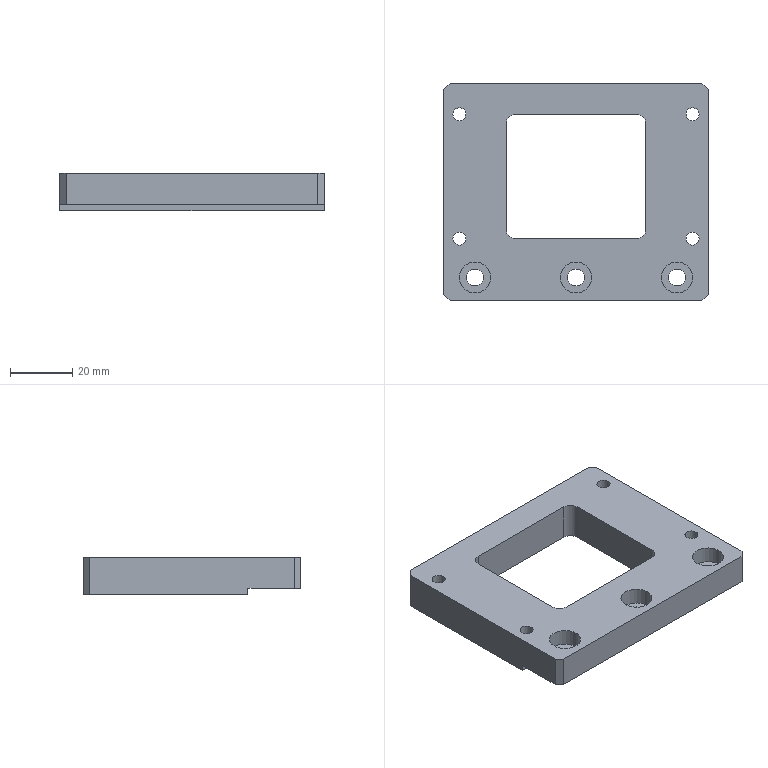Part | NX | 1 solid | 33 faces | box 85 x 70 x 12 mm | volume 44649 mm3 | plane 19 | cylinder 14 | commonest cylinder face diameters 4.2 x4 6 x4 5.5 x3 10 x3
STEP:
#1=CARTESIAN_POINT('',(-37.5,-27.5,0.6));
#2=VERTEX_POINT('',#1);
#3=CARTESIAN_POINT('',(-32.5,-27.5,0.6));
#4=DIRECTION('',(0.,0.,1.));
#5=DIRECTION('',(-1.,0.,0.));
#6=AXIS2_PLACEMENT_3D('',#3,#4,#5);
#7=CIRCLE('',#6,5.);
#8=EDGE_CURVE('',#2,#2,#7,.T.);
#9=ORIENTED_EDGE('',*,*,#8,.T.);
#10=EDGE_LOOP('',(#9));
#11=FACE_BOUND('',#10,.T.);
#12=CARTESIAN_POINT('',(-35.25,-27.5,0.6));
#13=VERTEX_POINT('',#12);
#14=CARTESIAN_POINT('',(-32.5,-27.5,0.6));
#15=DIRECTION('',(0.,0.,1.));
#16=DIRECTION('',(-1.,0.,0.));
#17=AXIS2_PLACEMENT_3D('',#14,#15,#16);
#18=CIRCLE('',#17,2.75);
#19=EDGE_CURVE('',#13,#13,#18,.T.);
#20=ORIENTED_EDGE('',*,*,#19,.F.);
#21=EDGE_LOOP('',(#20));
#22=FACE_BOUND('',#21,.T.);
#23=CARTESIAN_POINT('',(2.75,-27.5,0.6));
#24=DIRECTION('',(0.,0.,-1.));
#25=DIRECTION('',(-1.,0.,0.));
#26=AXIS2_PLACEMENT_3D('',#23,#24,#25);
#27=PLANE('',#26);
#28=ADVANCED_FACE('',(#11,#22),#27,.F.);
#29=CARTESIAN_POINT('',(5.,-27.5,0.6));
#30=VERTEX_POINT('',#29);
#31=CARTESIAN_POINT('',(0.,-27.5,0.6));
#32=DIRECTION('',(0.,0.,1.));
#33=DIRECTION('',(1.,0.,0.));
#34=AXIS2_PLACEMENT_3D('',#31,#32,#33);
#35=CIRCLE('',#34,5.);
#36=EDGE_CURVE('',#30,#30,#35,.T.);
#37=ORIENTED_EDGE('',*,*,#36,.T.);
#38=EDGE_LOOP('',(#37));
#39=FACE_BOUND('',#38,.T.);
#40=CARTESIAN_POINT('',(2.75,-27.5,0.6));
#41=VERTEX_POINT('',#40);
#42=CARTESIAN_POINT('',(0.,-27.5,0.6));
#43=DIRECTION('',(0.,0.,1.));
#44=DIRECTION('',(1.,0.,0.));
#45=AXIS2_PLACEMENT_3D('',#42,#43,#44);
#46=CIRCLE('',#45,2.75);
#47=EDGE_CURVE('',#41,#41,#46,.T.);
#48=ORIENTED_EDGE('',*,*,#47,.F.);
#49=EDGE_LOOP('',(#48));
#50=FACE_BOUND('',#49,.T.);
#51=CARTESIAN_POINT('',(2.75,-27.5,0.6));
#52=DIRECTION('',(0.,0.,-1.));
#53=DIRECTION('',(-1.,0.,0.));
#54=AXIS2_PLACEMENT_3D('',#51,#52,#53);
#55=PLANE('',#54);
#56=ADVANCED_FACE('',(#39,#50),#55,.F.);
#57=CARTESIAN_POINT('',(27.5,-27.5,0.6));
#58=VERTEX_POINT('',#57);
#59=CARTESIAN_POINT('',(32.5,-27.5,0.6));
#60=DIRECTION('',(0.,0.,1.));
#61=DIRECTION('',(-1.,0.,0.));
#62=AXIS2_PLACEMENT_3D('',#59,#60,#61);
#63=CIRCLE('',#62,5.);
#64=EDGE_CURVE('',#58,#58,#63,.T.);
#65=ORIENTED_EDGE('',*,*,#64,.T.);
#66=EDGE_LOOP('',(#65));
#67=FACE_BOUND('',#66,.T.);
#68=CARTESIAN_POINT('',(29.75,-27.5,0.6));
#69=VERTEX_POINT('',#68);
#70=CARTESIAN_POINT('',(32.5,-27.5,0.6));
#71=DIRECTION('',(0.,0.,1.));
#72=DIRECTION('',(-1.,0.,0.));
#73=AXIS2_PLACEMENT_3D('',#70,#71,#72);
#74=CIRCLE('',#73,2.75);
#75=EDGE_CURVE('',#69,#69,#74,.T.);
#76=ORIENTED_EDGE('',*,*,#75,.F.);
#77=EDGE_LOOP('',(#76));
#78=FACE_BOUND('',#77,.T.);
#79=CARTESIAN_POINT('',(2.75,-27.5,0.6));
#80=DIRECTION('',(0.,0.,-1.));
#81=DIRECTION('',(-1.,0.,0.));
#82=AXIS2_PLACEMENT_3D('',#79,#80,#81);
#83=PLANE('',#82);
#84=ADVANCED_FACE('',(#67,#78),#83,.F.);
#85=CARTESIAN_POINT('',(-19.5,-15.,6.));
#86=VERTEX_POINT('',#85);
#87=CARTESIAN_POINT('',(19.5,-15.,6.));
#88=VERTEX_POINT('',#87);
#89=CARTESIAN_POINT('',(19.5,-15.,6.));
#90=DIRECTION('',(1.,0.,0.));
#91=VECTOR('',#90,1000.);
#92=LINE('',#89,#91);
#93=EDGE_CURVE('',#86,#88,#92,.T.);
#94=ORIENTED_EDGE('',*,*,#93,.T.);
#95=CARTESIAN_POINT('',(19.5,-15.,-6.));
#96=VERTEX_POINT('',#95);
#97=CARTESIAN_POINT('',(19.5,-15.,-6.));
#98=DIRECTION('',(0.,0.,1.));
#99=VECTOR('',#98,1000.);
#100=LINE('',#97,#99);
#101=EDGE_CURVE('',#96,#88,#100,.T.);
#102=ORIENTED_EDGE('',*,*,#101,.F.);
#103=CARTESIAN_POINT('',(-19.5,-15.,-6.));
#104=VERTEX_POINT('',#103);
#105=CARTESIAN_POINT('',(19.5,-15.,-6.));
#106=DIRECTION('',(1.,0.,0.));
#107=VECTOR('',#106,1000.);
#108=LINE('',#105,#107);
#109=EDGE_CURVE('',#104,#96,#108,.T.);
#110=ORIENTED_EDGE('',*,*,#109,.F.);
#111=CARTESIAN_POINT('',(-19.5,-15.,-6.));
#112=DIRECTION('',(0.,0.,1.));
#113=VECTOR('',#112,1000.);
#114=LINE('',#111,#113);
#115=EDGE_CURVE('',#104,#86,#114,.T.);
#116=ORIENTED_EDGE('',*,*,#115,.T.);
#117=EDGE_LOOP('',(#94,#102,#110,#116));
#118=FACE_BOUND('',#117,.T.);
#119=CARTESIAN_POINT('',(19.5,-15.,-6.));
#120=DIRECTION('',(0.,-1.,0.));
#121=DIRECTION('',(1.,0.,0.));
#122=AXIS2_PLACEMENT_3D('',#119,#120,#121);
#123=PLANE('',#122);
#124=ADVANCED_FACE('',(#118),#123,.F.);
#125=CARTESIAN_POINT('',(22.5,-12.,6.));
#126=VERTEX_POINT('',#125);
#127=CARTESIAN_POINT('',(19.5,-12.,6.));
#128=DIRECTION('',(0.,0.,1.));
#129=DIRECTION('',(1.,0.,0.));
#130=AXIS2_PLACEMENT_3D('',#127,#128,#129);
#131=CIRCLE('',#130,3.);
#132=EDGE_CURVE('',#88,#126,#131,.T.);
#133=ORIENTED_EDGE('',*,*,#132,.T.);
#134=CARTESIAN_POINT('',(22.5,-12.,-6.));
#135=VERTEX_POINT('',#134);
#136=CARTESIAN_POINT('',(22.5,-12.,-6.));
#137=DIRECTION('',(0.,0.,1.));
#138=VECTOR('',#137,1000.);
#139=LINE('',#136,#138);
#140=EDGE_CURVE('',#135,#126,#139,.T.);
#141=ORIENTED_EDGE('',*,*,#140,.F.);
#142=CARTESIAN_POINT('',(19.5,-12.,-6.));
#143=DIRECTION('',(0.,0.,1.));
#144=DIRECTION('',(1.,0.,0.));
#145=AXIS2_PLACEMENT_3D('',#142,#143,#144);
#146=CIRCLE('',#145,3.);
#147=EDGE_CURVE('',#96,#135,#146,.T.);
#148=ORIENTED_EDGE('',*,*,#147,.F.);
#149=ORIENTED_EDGE('',*,*,#101,.T.);
#150=EDGE_LOOP('',(#133,#141,#148,#149));
#151=FACE_BOUND('',#150,.T.);
#152=CARTESIAN_POINT('',(19.5,-12.,-6.));
#153=DIRECTION('',(0.,0.,1.));
#154=DIRECTION('',(1.,0.,0.));
#155=AXIS2_PLACEMENT_3D('',#152,#153,#154);
#156=CYLINDRICAL_SURFACE('',#155,3.);
#157=ADVANCED_FACE('',(#151),#156,.F.);
#158=CARTESIAN_POINT('',(22.5,22.,6.));
#159=VERTEX_POINT('',#158);
#160=CARTESIAN_POINT('',(22.5,-12.,6.));
#161=DIRECTION('',(0.,1.,0.));
#162=VECTOR('',#161,1000.);
#163=LINE('',#160,#162);
#164=EDGE_CURVE('',#126,#159,#163,.T.);
#165=ORIENTED_EDGE('',*,*,#164,.T.);
#166=CARTESIAN_POINT('',(22.5,22.,-6.));
#167=VERTEX_POINT('',#166);
#168=CARTESIAN_POINT('',(22.5,22.,-6.));
#169=DIRECTION('',(0.,0.,1.));
#170=VECTOR('',#169,1000.);
#171=LINE('',#168,#170);
#172=EDGE_CURVE('',#167,#159,#171,.T.);
#173=ORIENTED_EDGE('',*,*,#172,.F.);
#174=CARTESIAN_POINT('',(22.5,-12.,-6.));
#175=DIRECTION('',(0.,1.,0.));
#176=VECTOR('',#175,1000.);
#177=LINE('',#174,#176);
#178=EDGE_CURVE('',#135,#167,#177,.T.);
#179=ORIENTED_EDGE('',*,*,#178,.F.);
#180=ORIENTED_EDGE('',*,*,#140,.T.);
#181=EDGE_LOOP('',(#165,#173,#179,#180));
#182=FACE_BOUND('',#181,.T.);
#183=CARTESIAN_POINT('',(22.5,-12.,-6.));
#184=DIRECTION('',(1.,0.,0.));
#185=DIRECTION('',(0.,0.,-1.));
#186=AXIS2_PLACEMENT_3D('',#183,#184,#185);
#187=PLANE('',#186);
#188=ADVANCED_FACE('',(#182),#187,.F.);
#189=CARTESIAN_POINT('',(19.5,25.,6.));
#190=VERTEX_POINT('',#189);
#191=CARTESIAN_POINT('',(19.5,22.,6.));
#192=DIRECTION('',(0.,0.,1.));
#193=DIRECTION('',(1.,0.,0.));
#194=AXIS2_PLACEMENT_3D('',#191,#192,#193);
#195=CIRCLE('',#194,3.);
#196=EDGE_CURVE('',#159,#190,#195,.T.);
#197=ORIENTED_EDGE('',*,*,#196,.T.);
#198=CARTESIAN_POINT('',(19.5,25.,-6.));
#199=VERTEX_POINT('',#198);
#200=CARTESIAN_POINT('',(19.5,25.,-6.));
#201=DIRECTION('',(0.,0.,1.));
#202=VECTOR('',#201,1000.);
#203=LINE('',#200,#202);
#204=EDGE_CURVE('',#199,#190,#203,.T.);
#205=ORIENTED_EDGE('',*,*,#204,.F.);
#206=CARTESIAN_POINT('',(19.5,22.,-6.));
#207=DIRECTION('',(0.,0.,1.));
#208=DIRECTION('',(1.,0.,0.));
#209=AXIS2_PLACEMENT_3D('',#206,#207,#208);
#210=CIRCLE('',#209,3.);
#211=EDGE_CURVE('',#167,#199,#210,.T.);
#212=ORIENTED_EDGE('',*,*,#211,.F.);
#213=ORIENTED_EDGE('',*,*,#172,.T.);
#214=EDGE_LOOP('',(#197,#205,#212,#213));
#215=FACE_BOUND('',#214,.T.);
#216=CARTESIAN_POINT('',(19.5,22.,-6.));
#217=DIRECTION('',(0.,0.,1.));
#218=DIRECTION('',(1.,0.,0.));
#219=AXIS2_PLACEMENT_3D('',#216,#217,#218);
#220=CYLINDRICAL_SURFACE('',#219,3.);
#221=ADVANCED_FACE('',(#215),#220,.F.);
#222=CARTESIAN_POINT('',(-19.5,25.,6.));
#223=VERTEX_POINT('',#222);
#224=CARTESIAN_POINT('',(19.5,25.,6.));
#225=DIRECTION('',(-1.,0.,0.));
#226=VECTOR('',#225,1000.);
#227=LINE('',#224,#226);
#228=EDGE_CURVE('',#190,#223,#227,.T.);
#229=ORIENTED_EDGE('',*,*,#228,.T.);
#230=CARTESIAN_POINT('',(-19.5,25.,-6.));
#231=VERTEX_POINT('',#230);
#232=CARTESIAN_POINT('',(-19.5,25.,-6.));
#233=DIRECTION('',(0.,0.,1.));
#234=VECTOR('',#233,1000.);
#235=LINE('',#232,#234);
#236=EDGE_CURVE('',#231,#223,#235,.T.);
#237=ORIENTED_EDGE('',*,*,#236,.F.);
#238=CARTESIAN_POINT('',(19.5,25.,-6.));
#239=DIRECTION('',(-1.,0.,0.));
#240=VECTOR('',#239,1000.);
#241=LINE('',#238,#240);
#242=EDGE_CURVE('',#199,#231,#241,.T.);
#243=ORIENTED_EDGE('',*,*,#242,.F.);
#244=ORIENTED_EDGE('',*,*,#204,.T.);
#245=EDGE_LOOP('',(#229,#237,#243,#244));
#246=FACE_BOUND('',#245,.T.);
#247=CARTESIAN_POINT('',(19.5,25.,-6.));
#248=DIRECTION('',(0.,1.,0.));
#249=DIRECTION('',(-1.,0.,0.));
#250=AXIS2_PLACEMENT_3D('',#247,#248,#249);
#251=PLANE('',#250);
#252=ADVANCED_FACE('',(#246),#251,.F.);
#253=CARTESIAN_POINT('',(-22.5,22.,6.));
#254=VERTEX_POINT('',#253);
#255=CARTESIAN_POINT('',(-19.5,22.,6.));
#256=DIRECTION('',(0.,0.,1.));
#257=DIRECTION('',(1.,0.,0.));
#258=AXIS2_PLACEMENT_3D('',#255,#256,#257);
#259=CIRCLE('',#258,3.);
#260=EDGE_CURVE('',#223,#254,#259,.T.);
#261=ORIENTED_EDGE('',*,*,#260,.T.);
#262=CARTESIAN_POINT('',(-22.5,22.,-6.));
#263=VERTEX_POINT('',#262);
#264=CARTESIAN_POINT('',(-22.5,22.,-6.));
#265=DIRECTION('',(0.,0.,1.));
#266=VECTOR('',#265,1000.);
#267=LINE('',#264,#266);
#268=EDGE_CURVE('',#263,#254,#267,.T.);
#269=ORIENTED_EDGE('',*,*,#268,.F.);
#270=CARTESIAN_POINT('',(-19.5,22.,-6.));
#271=DIRECTION('',(0.,0.,1.));
#272=DIRECTION('',(1.,0.,0.));
#273=AXIS2_PLACEMENT_3D('',#270,#271,#272);
#274=CIRCLE('',#273,3.);
#275=EDGE_CURVE('',#231,#263,#274,.T.);
#276=ORIENTED_EDGE('',*,*,#275,.F.);
#277=ORIENTED_EDGE('',*,*,#236,.T.);
#278=EDGE_LOOP('',(#261,#269,#276,#277));
#279=FACE_BOUND('',#278,.T.);
#280=CARTESIAN_POINT('',(-19.5,22.,-6.));
#281=DIRECTION('',(0.,0.,1.));
#282=DIRECTION('',(1.,0.,0.));
#283=AXIS2_PLACEMENT_3D('',#280,#281,#282);
#284=CYLINDRICAL_SURFACE('',#283,3.);
#285=ADVANCED_FACE('',(#279),#284,.F.);
#286=CARTESIAN_POINT('',(-22.5,-12.,6.));
#287=VERTEX_POINT('',#286);
#288=CARTESIAN_POINT('',(-22.5,-12.,6.));
#289=DIRECTION('',(0.,-1.,0.));
#290=VECTOR('',#289,1000.);
#291=LINE('',#288,#290);
#292=EDGE_CURVE('',#254,#287,#291,.T.);
#293=ORIENTED_EDGE('',*,*,#292,.T.);
#294=CARTESIAN_POINT('',(-22.5,-12.,-6.));
#295=VERTEX_POINT('',#294);
#296=CARTESIAN_POINT('',(-22.5,-12.,-6.));
#297=DIRECTION('',(0.,0.,1.));
#298=VECTOR('',#297,1000.);
#299=LINE('',#296,#298);
#300=EDGE_CURVE('',#295,#287,#299,.T.);
#301=ORIENTED_EDGE('',*,*,#300,.F.);
#302=CARTESIAN_POINT('',(-22.5,-12.,-6.));
#303=DIRECTION('',(0.,-1.,0.));
#304=VECTOR('',#303,1000.);
#305=LINE('',#302,#304);
#306=EDGE_CURVE('',#263,#295,#305,.T.);
#307=ORIENTED_EDGE('',*,*,#306,.F.);
#308=ORIENTED_EDGE('',*,*,#268,.T.);
#309=EDGE_LOOP('',(#293,#301,#307,#308));
#310=FACE_BOUND('',#309,.T.);
#311=CARTESIAN_POINT('',(-22.5,-12.,-6.));
#312=DIRECTION('',(-1.,0.,0.));
#313=DIRECTION('',(0.,0.,1.));
#314=AXIS2_PLACEMENT_3D('',#311,#312,#313);
#315=PLANE('',#314);
#316=ADVANCED_FACE('',(#310),#315,.F.);
#317=CARTESIAN_POINT('',(-19.5,-12.,6.));
#318=DIRECTION('',(0.,0.,1.));
#319=DIRECTION('',(-1.,0.,0.));
#320=AXIS2_PLACEMENT_3D('',#317,#318,#319);
#321=CIRCLE('',#320,3.);
#322=EDGE_CURVE('',#287,#86,#321,.T.);
#323=ORIENTED_EDGE('',*,*,#322,.T.);
#324=ORIENTED_EDGE('',*,*,#115,.F.);
#325=CARTESIAN_POINT('',(-19.5,-12.,-6.));
#326=DIRECTION('',(0.,0.,1.));
#327=DIRECTION('',(-1.,0.,0.));
#328=AXIS2_PLACEMENT_3D('',#325,#326,#327);
#329=CIRCLE('',#328,3.);
#330=EDGE_CURVE('',#295,#104,#329,.T.);
#331=ORIENTED_EDGE('',*,*,#330,.F.);
#332=ORIENTED_EDGE('',*,*,#300,.T.);
#333=EDGE_LOOP('',(#323,#324,#331,#332));
#334=FACE_BOUND('',#333,.T.);
#335=CARTESIAN_POINT('',(-19.5,-12.,-6.));
#336=DIRECTION('',(0.,0.,1.));
#337=DIRECTION('',(1.,0.,0.));
#338=AXIS2_PLACEMENT_3D('',#335,#336,#337);
#339=CYLINDRICAL_SURFACE('',#338,3.);
#340=ADVANCED_FACE('',(#334),#339,.F.);
#341=CARTESIAN_POINT('',(42.5,33.,6.));
#342=VERTEX_POINT('',#341);
#343=CARTESIAN_POINT('',(40.5,35.,6.));
#344=VERTEX_POINT('',#343);
#345=CARTESIAN_POINT('',(37.75,37.75,6.));
#346=DIRECTION('',(-0.7071,0.7071,0.));
#347=VECTOR('',#346,1000.);
#348=LINE('',#345,#347);
#349=EDGE_CURVE('',#342,#344,#348,.T.);
#350=ORIENTED_EDGE('',*,*,#349,.F.);
#351=CARTESIAN_POINT('',(42.5,33.,-6.));
#352=VERTEX_POINT('',#351);
#353=CARTESIAN_POINT('',(42.5,33.,6.));
#354=DIRECTION('',(0.,0.,1.));
#355=VECTOR('',#354,1000.);
#356=LINE('',#353,#355);
#357=EDGE_CURVE('',#352,#342,#356,.T.);
#358=ORIENTED_EDGE('',*,*,#357,.F.);
#359=CARTESIAN_POINT('',(40.5,35.,-6.));
#360=VERTEX_POINT('',#359);
#361=CARTESIAN_POINT('',(40.5,35.,-6.));
#362=DIRECTION('',(0.7071,-0.7071,0.));
#363=VECTOR('',#362,1000.);
#364=LINE('',#361,#363);
#365=EDGE_CURVE('',#360,#352,#364,.T.);
#366=ORIENTED_EDGE('',*,*,#365,.F.);
#367=CARTESIAN_POINT('',(40.5,35.,6.));
#368=DIRECTION('',(0.,0.,-1.));
#369=VECTOR('',#368,1000.);
#370=LINE('',#367,#369);
#371=EDGE_CURVE('',#344,#360,#370,.T.);
#372=ORIENTED_EDGE('',*,*,#371,.F.);
#373=EDGE_LOOP('',(#350,#358,#366,#372));
#374=FACE_BOUND('',#373,.T.);
#375=CARTESIAN_POINT('',(40.5,35.,6.));
#376=DIRECTION('',(-0.7071,-0.7071,0.));
#377=DIRECTION('',(0.,0.,-1.));
#378=AXIS2_PLACEMENT_3D('',#375,#376,#377);
#379=PLANE('',#378);
#380=ADVANCED_FACE('',(#374),#379,.F.);
#381=CARTESIAN_POINT('',(-40.5,35.,6.));
#382=VERTEX_POINT('',#381);
#383=CARTESIAN_POINT('',(-42.5,33.,6.));
#384=VERTEX_POINT('',#383);
#385=CARTESIAN_POINT('',(-37.75,37.75,6.));
#386=DIRECTION('',(-0.7071,-0.7071,0.));
#387=VECTOR('',#386,1000.);
#388=LINE('',#385,#387);
#389=EDGE_CURVE('',#382,#384,#388,.T.);
#390=ORIENTED_EDGE('',*,*,#389,.F.);
#391=CARTESIAN_POINT('',(-40.5,35.,-6.));
#392=VERTEX_POINT('',#391);
#393=CARTESIAN_POINT('',(-40.5,35.,6.));
#394=DIRECTION('',(0.,0.,1.));
#395=VECTOR('',#394,1000.);
#396=LINE('',#393,#395);
#397=EDGE_CURVE('',#392,#382,#396,.T.);
#398=ORIENTED_EDGE('',*,*,#397,.F.);
#399=CARTESIAN_POINT('',(-42.5,33.,-6.));
#400=VERTEX_POINT('',#399);
#401=CARTESIAN_POINT('',(-42.5,33.,-6.));
#402=DIRECTION('',(0.7071,0.7071,0.));
#403=VECTOR('',#402,1000.);
#404=LINE('',#401,#403);
#405=EDGE_CURVE('',#400,#392,#404,.T.);
#406=ORIENTED_EDGE('',*,*,#405,.F.);
#407=CARTESIAN_POINT('',(-42.5,33.,6.));
#408=DIRECTION('',(0.,0.,-1.));
#409=VECTOR('',#408,1000.);
#410=LINE('',#407,#409);
#411=EDGE_CURVE('',#384,#400,#410,.T.);
#412=ORIENTED_EDGE('',*,*,#411,.F.);
#413=EDGE_LOOP('',(#390,#398,#406,#412));
#414=FACE_BOUND('',#413,.T.);
#415=CARTESIAN_POINT('',(-42.5,33.,6.));
#416=DIRECTION('',(0.7071,-0.7071,0.));
#417=DIRECTION('',(0.,0.,-1.));
#418=AXIS2_PLACEMENT_3D('',#415,#416,#417);
#419=PLANE('',#418);
#420=ADVANCED_FACE('',(#414),#419,.F.);
#421=CARTESIAN_POINT('',(-42.5,-33.,6.));
#422=VERTEX_POINT('',#421);
#423=CARTESIAN_POINT('',(-40.5,-35.,6.));
#424=VERTEX_POINT('',#423);
#425=CARTESIAN_POINT('',(-37.75,-37.75,6.));
#426=DIRECTION('',(0.7071,-0.7071,0.));
#427=VECTOR('',#426,1000.);
#428=LINE('',#425,#427);
#429=EDGE_CURVE('',#422,#424,#428,.T.);
#430=ORIENTED_EDGE('',*,*,#429,.F.);
#431=CARTESIAN_POINT('',(-42.5,-33.,-4.));
#432=VERTEX_POINT('',#431);
#433=CARTESIAN_POINT('',(-42.5,-33.,6.));
#434=DIRECTION('',(0.,0.,1.));
#435=VECTOR('',#434,1000.);
#436=LINE('',#433,#435);
#437=EDGE_CURVE('',#432,#422,#436,.T.);
#438=ORIENTED_EDGE('',*,*,#437,.F.);
#439=CARTESIAN_POINT('',(-40.5,-35.,-4.));
#440=VERTEX_POINT('',#439);
#441=CARTESIAN_POINT('',(-40.5,-35.,-4.));
#442=DIRECTION('',(-0.7071,0.7071,0.));
#443=VECTOR('',#442,1000.);
#444=LINE('',#441,#443);
#445=EDGE_CURVE('',#440,#432,#444,.T.);
#446=ORIENTED_EDGE('',*,*,#445,.F.);
#447=CARTESIAN_POINT('',(-40.5,-35.,6.));
#448=DIRECTION('',(0.,0.,-1.));
#449=VECTOR('',#448,1000.);
#450=LINE('',#447,#449);
#451=EDGE_CURVE('',#424,#440,#450,.T.);
#452=ORIENTED_EDGE('',*,*,#451,.F.);
#453=EDGE_LOOP('',(#430,#438,#446,#452));
#454=FACE_BOUND('',#453,.T.);
#455=CARTESIAN_POINT('',(-40.5,-35.,6.));
#456=DIRECTION('',(0.7071,0.7071,0.));
#457=DIRECTION('',(0.,0.,-1.));
#458=AXIS2_PLACEMENT_3D('',#455,#456,#457);
#459=PLANE('',#458);
#460=ADVANCED_FACE('',(#454),#459,.F.);
#461=CARTESIAN_POINT('',(40.5,-35.,6.));
#462=VERTEX_POINT('',#461);
#463=CARTESIAN_POINT('',(42.5,-33.,6.));
#464=VERTEX_POINT('',#463);
#465=CARTESIAN_POINT('',(37.75,-37.75,6.));
#466=DIRECTION('',(0.7071,0.7071,0.));
#467=VECTOR('',#466,1000.);
#468=LINE('',#465,#467);
#469=EDGE_CURVE('',#462,#464,#468,.T.);
#470=ORIENTED_EDGE('',*,*,#469,.F.);
#471=CARTESIAN_POINT('',(40.5,-35.,-4.));
#472=VERTEX_POINT('',#471);
#473=CARTESIAN_POINT('',(40.5,-35.,6.));
#474=DIRECTION('',(0.,0.,1.));
#475=VECTOR('',#474,1000.);
#476=LINE('',#473,#475);
#477=EDGE_CURVE('',#472,#462,#476,.T.);
#478=ORIENTED_EDGE('',*,*,#477,.F.);
#479=CARTESIAN_POINT('',(42.5,-33.,-4.));
#480=VERTEX_POINT('',#479);
#481=CARTESIAN_POINT('',(42.5,-33.,-4.));
#482=DIRECTION('',(-0.7071,-0.7071,0.));
#483=VECTOR('',#482,1000.);
#484=LINE('',#481,#483);
#485=EDGE_CURVE('',#480,#472,#484,.T.);
#486=ORIENTED_EDGE('',*,*,#485,.F.);
#487=CARTESIAN_POINT('',(42.5,-33.,6.));
#488=DIRECTION('',(0.,0.,-1.));
#489=VECTOR('',#488,1000.);
#490=LINE('',#487,#489);
#491=EDGE_CURVE('',#464,#480,#490,.T.);
#492=ORIENTED_EDGE('',*,*,#491,.F.);
#493=EDGE_LOOP('',(#470,#478,#486,#492));
#494=FACE_BOUND('',#493,.T.);
#495=CARTESIAN_POINT('',(42.5,-33.,6.));
#496=DIRECTION('',(-0.7071,0.7071,0.));
#497=DIRECTION('',(0.,0.,-1.));
#498=AXIS2_PLACEMENT_3D('',#495,#496,#497);
#499=PLANE('',#498);
#500=ADVANCED_FACE('',(#494),#499,.F.);
#501=CARTESIAN_POINT('',(42.5,-18.,-4.));
#502=VERTEX_POINT('',#501);
#503=CARTESIAN_POINT('',(42.5,-35.,-4.));
#504=DIRECTION('',(0.,-1.,0.));
#505=VECTOR('',#504,1000.);
#506=LINE('',#503,#505);
#507=EDGE_CURVE('',#502,#480,#506,.T.);
#508=ORIENTED_EDGE('',*,*,#507,.T.);
#509=ORIENTED_EDGE('',*,*,#485,.T.);
#510=CARTESIAN_POINT('',(42.5,-35.,-4.));
#511=DIRECTION('',(-1.,0.,0.));
#512=VECTOR('',#511,1000.);
#513=LINE('',#510,#512);
#514=EDGE_CURVE('',#472,#440,#513,.T.);
#515=ORIENTED_EDGE('',*,*,#514,.T.);
#516=ORIENTED_EDGE('',*,*,#445,.T.);
#517=CARTESIAN_POINT('',(-42.5,-18.,-4.));
#518=VERTEX_POINT('',#517);
#519=CARTESIAN_POINT('',(-42.5,-35.,-4.));
#520=DIRECTION('',(0.,1.,0.));
#521=VECTOR('',#520,1000.);
#522=LINE('',#519,#521);
#523=EDGE_CURVE('',#432,#518,#522,.T.);
#524=ORIENTED_EDGE('',*,*,#523,.T.);
#525=CARTESIAN_POINT('',(42.5,-18.,-4.));
#526=DIRECTION('',(1.,0.,0.));
#527=VECTOR('',#526,1000.);
#528=LINE('',#525,#527);
#529=EDGE_CURVE('',#518,#502,#528,.T.);
#530=ORIENTED_EDGE('',*,*,#529,.T.);
#531=EDGE_LOOP('',(#508,#509,#515,#516,#524,#530));
#532=FACE_BOUND('',#531,.T.);
#533=CARTESIAN_POINT('',(35.25,-27.5,-4.));
#534=VERTEX_POINT('',#533);
#535=CARTESIAN_POINT('',(32.5,-27.5,-4.));
#536=DIRECTION('',(0.,0.,1.));
#537=DIRECTION('',(1.,0.,0.));
#538=AXIS2_PLACEMENT_3D('',#535,#536,#537);
#539=CIRCLE('',#538,2.75);
#540=EDGE_CURVE('',#534,#534,#539,.T.);
#541=ORIENTED_EDGE('',*,*,#540,.T.);
#542=EDGE_LOOP('',(#541));
#543=FACE_BOUND('',#542,.T.);
#544=CARTESIAN_POINT('',(2.75,-27.5,-4.));
#545=VERTEX_POINT('',#544);
#546=CARTESIAN_POINT('',(0.,-27.5,-4.));
#547=DIRECTION('',(0.,0.,1.));
#548=DIRECTION('',(1.,0.,0.));
#549=AXIS2_PLACEMENT_3D('',#546,#547,#548);
#550=CIRCLE('',#549,2.75);
#551=EDGE_CURVE('',#545,#545,#550,.T.);
#552=ORIENTED_EDGE('',*,*,#551,.T.);
#553=EDGE_LOOP('',(#552));
#554=FACE_BOUND('',#553,.T.);
#555=CARTESIAN_POINT('',(-29.75,-27.5,-4.));
#556=VERTEX_POINT('',#555);
#557=CARTESIAN_POINT('',(-32.5,-27.5,-4.));
#558=DIRECTION('',(0.,0.,1.));
#559=DIRECTION('',(1.,0.,0.));
#560=AXIS2_PLACEMENT_3D('',#557,#558,#559);
#561=CIRCLE('',#560,2.75);
#562=EDGE_CURVE('',#556,#556,#561,.T.);
#563=ORIENTED_EDGE('',*,*,#562,.T.);
#564=EDGE_LOOP('',(#563));
#565=FACE_BOUND('',#564,.T.);
#566=CARTESIAN_POINT('',(0.,0.,-4.));
#567=DIRECTION('',(0.,0.,1.));
#568=DIRECTION('',(1.,0.,0.));
#569=AXIS2_PLACEMENT_3D('',#566,#567,#568);
#570=PLANE('',#569);
#571=ADVANCED_FACE('',(#532,#543,#554,#565),#570,.F.);
#572=CARTESIAN_POINT('',(-42.5,-18.,-6.));
#573=VERTEX_POINT('',#572);
#574=CARTESIAN_POINT('',(42.5,-18.,-6.));
#575=VERTEX_POINT('',#574);
#576=CARTESIAN_POINT('',(42.5,-18.,-6.));
#577=DIRECTION('',(1.,0.,0.));
#578=VECTOR('',#577,1000.);
#579=LINE('',#576,#578);
#580=EDGE_CURVE('',#573,#575,#579,.T.);
#581=ORIENTED_EDGE('',*,*,#580,.T.);
#582=CARTESIAN_POINT('',(42.5,-18.,-4.));
#583=DIRECTION('',(0.,0.,-1.));
#584=VECTOR('',#583,1000.);
#585=LINE('',#582,#584);
#586=EDGE_CURVE('',#502,#575,#585,.T.);
#587=ORIENTED_EDGE('',*,*,#586,.F.);
#588=ORIENTED_EDGE('',*,*,#529,.F.);
#589=CARTESIAN_POINT('',(-42.5,-18.,-4.));
#590=DIRECTION('',(0.,0.,-1.));
#591=VECTOR('',#590,1000.);
#592=LINE('',#589,#591);
#593=EDGE_CURVE('',#518,#573,#592,.T.);
#594=ORIENTED_EDGE('',*,*,#593,.T.);
#595=EDGE_LOOP('',(#581,#587,#588,#594));
#596=FACE_BOUND('',#595,.T.);
#597=CARTESIAN_POINT('',(42.5,-18.,-4.));
#598=DIRECTION('',(0.,1.,0.));
#599=DIRECTION('',(0.,0.,1.));
#600=AXIS2_PLACEMENT_3D('',#597,#598,#599);
#601=PLANE('',#600);
#602=ADVANCED_FACE('',(#596),#601,.F.);
#603=CARTESIAN_POINT('',(-42.5,35.,-6.));
#604=DIRECTION('',(0.,-1.,0.));
#605=VECTOR('',#604,1000.);
#606=LINE('',#603,#605);
#607=EDGE_CURVE('',#400,#573,#606,.T.);
#608=ORIENTED_EDGE('',*,*,#607,.F.);
#609=ORIENTED_EDGE('',*,*,#405,.T.);
#610=CARTESIAN_POINT('',(-42.5,35.,-6.));
#611=DIRECTION('',(-1.,0.,0.));
#612=VECTOR('',#611,1000.);
#613=LINE('',#610,#612);
#614=EDGE_CURVE('',#360,#392,#613,.T.);
#615=ORIENTED_EDGE('',*,*,#614,.F.);
#616=ORIENTED_EDGE('',*,*,#365,.T.);
#617=CARTESIAN_POINT('',(42.5,35.,-6.));
#618=DIRECTION('',(0.,1.,0.));
#619=VECTOR('',#618,1000.);
#620=LINE('',#617,#619);
#621=EDGE_CURVE('',#575,#352,#620,.T.);
#622=ORIENTED_EDGE('',*,*,#621,.F.);
#623=ORIENTED_EDGE('',*,*,#580,.F.);
#624=EDGE_LOOP('',(#608,#609,#615,#616,#622,#623));
#625=FACE_BOUND('',#624,.T.);
#626=ORIENTED_EDGE('',*,*,#306,.T.);
#627=ORIENTED_EDGE('',*,*,#330,.T.);
#628=ORIENTED_EDGE('',*,*,#109,.T.);
#629=ORIENTED_EDGE('',*,*,#147,.T.);
#630=ORIENTED_EDGE('',*,*,#178,.T.);
#631=ORIENTED_EDGE('',*,*,#211,.T.);
#632=ORIENTED_EDGE('',*,*,#242,.T.);
#633=ORIENTED_EDGE('',*,*,#275,.T.);
#634=EDGE_LOOP('',(#626,#627,#628,#629,#630,#631,#632,#633));
#635=FACE_BOUND('',#634,.T.);
#636=CARTESIAN_POINT('',(39.6,25.,-6.));
#637=VERTEX_POINT('',#636);
#638=CARTESIAN_POINT('',(37.5,25.,-6.));
#639=DIRECTION('',(0.,0.,1.));
#640=DIRECTION('',(1.,0.,0.));
#641=AXIS2_PLACEMENT_3D('',#638,#639,#640);
#642=CIRCLE('',#641,2.1);
#643=EDGE_CURVE('',#637,#637,#642,.T.);
#644=ORIENTED_EDGE('',*,*,#643,.T.);
#645=EDGE_LOOP('',(#644));
#646=FACE_BOUND('',#645,.T.);
#647=CARTESIAN_POINT('',(39.6,-15.,-6.));
#648=VERTEX_POINT('',#647);
#649=CARTESIAN_POINT('',(37.5,-15.,-6.));
#650=DIRECTION('',(0.,0.,1.));
#651=DIRECTION('',(1.,0.,0.));
#652=AXIS2_PLACEMENT_3D('',#649,#650,#651);
#653=CIRCLE('',#652,2.1);
#654=EDGE_CURVE('',#648,#648,#653,.T.);
#655=ORIENTED_EDGE('',*,*,#654,.T.);
#656=EDGE_LOOP('',(#655));
#657=FACE_BOUND('',#656,.T.);
#658=CARTESIAN_POINT('',(-35.4,-15.,-6.));
#659=VERTEX_POINT('',#658);
#660=CARTESIAN_POINT('',(-37.5,-15.,-6.));
#661=DIRECTION('',(0.,0.,1.));
#662=DIRECTION('',(1.,0.,0.));
#663=AXIS2_PLACEMENT_3D('',#660,#661,#662);
#664=CIRCLE('',#663,2.1);
#665=EDGE_CURVE('',#659,#659,#664,.T.);
#666=ORIENTED_EDGE('',*,*,#665,.T.);
#667=EDGE_LOOP('',(#666));
#668=FACE_BOUND('',#667,.T.);
#669=CARTESIAN_POINT('',(-35.4,25.,-6.));
#670=VERTEX_POINT('',#669);
#671=CARTESIAN_POINT('',(-37.5,25.,-6.));
#672=DIRECTION('',(0.,0.,1.));
#673=DIRECTION('',(1.,0.,0.));
#674=AXIS2_PLACEMENT_3D('',#671,#672,#673);
#675=CIRCLE('',#674,2.1);
#676=EDGE_CURVE('',#670,#670,#675,.T.);
#677=ORIENTED_EDGE('',*,*,#676,.T.);
#678=EDGE_LOOP('',(#677));
#679=FACE_BOUND('',#678,.T.);
#680=CARTESIAN_POINT('',(0.,0.,-6.));
#681=DIRECTION('',(0.,0.,1.));
#682=DIRECTION('',(1.,0.,0.));
#683=AXIS2_PLACEMENT_3D('',#680,#681,#682);
#684=PLANE('',#683);
#685=ADVANCED_FACE('',(#625,#635,#646,#657,#668,#679),#684,.F.);
#686=CARTESIAN_POINT('',(-42.5,-35.,6.));
#687=DIRECTION('',(1.,0.,0.));
#688=VECTOR('',#687,1000.);
#689=LINE('',#686,#688);
#690=EDGE_CURVE('',#424,#462,#689,.T.);
#691=ORIENTED_EDGE('',*,*,#690,.T.);
#692=ORIENTED_EDGE('',*,*,#469,.T.);
#693=CARTESIAN_POINT('',(42.5,35.,6.));
#694=DIRECTION('',(0.,1.,0.));
#695=VECTOR('',#694,1000.);
#696=LINE('',#693,#695);
#697=EDGE_CURVE('',#464,#342,#696,.T.);
#698=ORIENTED_EDGE('',*,*,#697,.T.);
#699=ORIENTED_EDGE('',*,*,#349,.T.);
#700=CARTESIAN_POINT('',(-42.5,35.,6.));
#701=DIRECTION('',(-1.,0.,0.));
#702=VECTOR('',#701,1000.);
#703=LINE('',#700,#702);
#704=EDGE_CURVE('',#344,#382,#703,.T.);
#705=ORIENTED_EDGE('',*,*,#704,.T.);
#706=ORIENTED_EDGE('',*,*,#389,.T.);
#707=CARTESIAN_POINT('',(-42.5,35.,6.));
#708=DIRECTION('',(0.,-1.,0.));
#709=VECTOR('',#708,1000.);
#710=LINE('',#707,#709);
#711=EDGE_CURVE('',#384,#422,#710,.T.);
#712=ORIENTED_EDGE('',*,*,#711,.T.);
#713=ORIENTED_EDGE('',*,*,#429,.T.);
#714=EDGE_LOOP('',(#691,#692,#698,#699,#705,#706,#712,#713));
#715=FACE_BOUND('',#714,.T.);
#716=ORIENTED_EDGE('',*,*,#322,.F.);
#717=ORIENTED_EDGE('',*,*,#292,.F.);
#718=ORIENTED_EDGE('',*,*,#260,.F.);
#719=ORIENTED_EDGE('',*,*,#228,.F.);
#720=ORIENTED_EDGE('',*,*,#196,.F.);
#721=ORIENTED_EDGE('',*,*,#164,.F.);
#722=ORIENTED_EDGE('',*,*,#132,.F.);
#723=ORIENTED_EDGE('',*,*,#93,.F.);
#724=EDGE_LOOP('',(#716,#717,#718,#719,#720,#721,#722,#723));
#725=FACE_BOUND('',#724,.T.);
#726=CARTESIAN_POINT('',(37.5,-27.5,6.));
#727=VERTEX_POINT('',#726);
#728=CARTESIAN_POINT('',(32.5,-27.5,6.));
#729=DIRECTION('',(0.,0.,1.));
#730=DIRECTION('',(1.,0.,0.));
#731=AXIS2_PLACEMENT_3D('',#728,#729,#730);
#732=CIRCLE('',#731,5.);
#733=EDGE_CURVE('',#727,#727,#732,.T.);
#734=ORIENTED_EDGE('',*,*,#733,.F.);
#735=EDGE_LOOP('',(#734));
#736=FACE_BOUND('',#735,.T.);
#737=CARTESIAN_POINT('',(5.,-27.5,6.));
#738=VERTEX_POINT('',#737);
#739=CARTESIAN_POINT('',(0.,-27.5,6.));
#740=DIRECTION('',(0.,0.,1.));
#741=DIRECTION('',(1.,0.,0.));
#742=AXIS2_PLACEMENT_3D('',#739,#740,#741);
#743=CIRCLE('',#742,5.);
#744=EDGE_CURVE('',#738,#738,#743,.T.);
#745=ORIENTED_EDGE('',*,*,#744,.F.);
#746=EDGE_LOOP('',(#745));
#747=FACE_BOUND('',#746,.T.);
#748=CARTESIAN_POINT('',(-27.5,-27.5,6.));
#749=VERTEX_POINT('',#748);
#750=CARTESIAN_POINT('',(-32.5,-27.5,6.));
#751=DIRECTION('',(0.,0.,1.));
#752=DIRECTION('',(1.,0.,0.));
#753=AXIS2_PLACEMENT_3D('',#750,#751,#752);
#754=CIRCLE('',#753,5.);
#755=EDGE_CURVE('',#749,#749,#754,.T.);
#756=ORIENTED_EDGE('',*,*,#755,.F.);
#757=EDGE_LOOP('',(#756));
#758=FACE_BOUND('',#757,.T.);
#759=CARTESIAN_POINT('',(39.6,25.,6.));
#760=VERTEX_POINT('',#759);
#761=CARTESIAN_POINT('',(37.5,25.,6.));
#762=DIRECTION('',(0.,0.,1.));
#763=DIRECTION('',(1.,0.,0.));
#764=AXIS2_PLACEMENT_3D('',#761,#762,#763);
#765=CIRCLE('',#764,2.1);
#766=EDGE_CURVE('',#760,#760,#765,.T.);
#767=ORIENTED_EDGE('',*,*,#766,.F.);
#768=EDGE_LOOP('',(#767));
#769=FACE_BOUND('',#768,.T.);
#770=CARTESIAN_POINT('',(39.6,-15.,6.));
#771=VERTEX_POINT('',#770);
#772=CARTESIAN_POINT('',(37.5,-15.,6.));
#773=DIRECTION('',(0.,0.,1.));
#774=DIRECTION('',(1.,0.,0.));
#775=AXIS2_PLACEMENT_3D('',#772,#773,#774);
#776=CIRCLE('',#775,2.1);
#777=EDGE_CURVE('',#771,#771,#776,.T.);
#778=ORIENTED_EDGE('',*,*,#777,.F.);
#779=EDGE_LOOP('',(#778));
#780=FACE_BOUND('',#779,.T.);
#781=CARTESIAN_POINT('',(-35.4,-15.,6.));
#782=VERTEX_POINT('',#781);
#783=CARTESIAN_POINT('',(-37.5,-15.,6.));
#784=DIRECTION('',(0.,0.,1.));
#785=DIRECTION('',(1.,0.,0.));
#786=AXIS2_PLACEMENT_3D('',#783,#784,#785);
#787=CIRCLE('',#786,2.1);
#788=EDGE_CURVE('',#782,#782,#787,.T.);
#789=ORIENTED_EDGE('',*,*,#788,.F.);
#790=EDGE_LOOP('',(#789));
#791=FACE_BOUND('',#790,.T.);
#792=CARTESIAN_POINT('',(-35.4,25.,6.));
#793=VERTEX_POINT('',#792);
#794=CARTESIAN_POINT('',(-37.5,25.,6.));
#795=DIRECTION('',(0.,0.,1.));
#796=DIRECTION('',(1.,0.,0.));
#797=AXIS2_PLACEMENT_3D('',#794,#795,#796);
#798=CIRCLE('',#797,2.1);
#799=EDGE_CURVE('',#793,#793,#798,.T.);
#800=ORIENTED_EDGE('',*,*,#799,.F.);
#801=EDGE_LOOP('',(#800));
#802=FACE_BOUND('',#801,.T.);
#803=CARTESIAN_POINT('',(0.,0.,6.));
#804=DIRECTION('',(0.,0.,1.));
#805=DIRECTION('',(1.,0.,0.));
#806=AXIS2_PLACEMENT_3D('',#803,#804,#805);
#807=PLANE('',#806);
#808=ADVANCED_FACE('',(#715,#725,#736,#747,#758,#769,#780,#791,#802),#807,.T.);
#809=ORIENTED_EDGE('',*,*,#514,.F.);
#810=ORIENTED_EDGE('',*,*,#477,.T.);
#811=ORIENTED_EDGE('',*,*,#690,.F.);
#812=ORIENTED_EDGE('',*,*,#451,.T.);
#813=EDGE_LOOP('',(#809,#810,#811,#812));
#814=FACE_BOUND('',#813,.T.);
#815=CARTESIAN_POINT('',(-42.5,-35.,6.));
#816=DIRECTION('',(0.,1.,0.));
#817=DIRECTION('',(0.,0.,1.));
#818=AXIS2_PLACEMENT_3D('',#815,#816,#817);
#819=PLANE('',#818);
#820=ADVANCED_FACE('',(#814),#819,.F.);
#821=ORIENTED_EDGE('',*,*,#523,.F.);
#822=ORIENTED_EDGE('',*,*,#437,.T.);
#823=ORIENTED_EDGE('',*,*,#711,.F.);
#824=ORIENTED_EDGE('',*,*,#411,.T.);
#825=ORIENTED_EDGE('',*,*,#607,.T.);
#826=ORIENTED_EDGE('',*,*,#593,.F.);
#827=EDGE_LOOP('',(#821,#822,#823,#824,#825,#826));
#828=FACE_BOUND('',#827,.T.);
#829=CARTESIAN_POINT('',(-42.5,35.,6.));
#830=DIRECTION('',(1.,0.,0.));
#831=DIRECTION('',(0.,1.,0.));
#832=AXIS2_PLACEMENT_3D('',#829,#830,#831);
#833=PLANE('',#832);
#834=ADVANCED_FACE('',(#828),#833,.F.);
#835=ORIENTED_EDGE('',*,*,#614,.T.);
#836=ORIENTED_EDGE('',*,*,#397,.T.);
#837=ORIENTED_EDGE('',*,*,#704,.F.);
#838=ORIENTED_EDGE('',*,*,#371,.T.);
#839=EDGE_LOOP('',(#835,#836,#837,#838));
#840=FACE_BOUND('',#839,.T.);
#841=CARTESIAN_POINT('',(-42.5,35.,6.));
#842=DIRECTION('',(0.,-1.,0.));
#843=DIRECTION('',(0.,0.,-1.));
#844=AXIS2_PLACEMENT_3D('',#841,#842,#843);
#845=PLANE('',#844);
#846=ADVANCED_FACE('',(#840),#845,.F.);
#847=ORIENTED_EDGE('',*,*,#697,.F.);
#848=ORIENTED_EDGE('',*,*,#491,.T.);
#849=ORIENTED_EDGE('',*,*,#507,.F.);
#850=ORIENTED_EDGE('',*,*,#586,.T.);
#851=ORIENTED_EDGE('',*,*,#621,.T.);
#852=ORIENTED_EDGE('',*,*,#357,.T.);
#853=EDGE_LOOP('',(#847,#848,#849,#850,#851,#852));
#854=FACE_BOUND('',#853,.T.);
#855=CARTESIAN_POINT('',(42.5,35.,6.));
#856=DIRECTION('',(-1.,0.,0.));
#857=DIRECTION('',(0.,-1.,0.));
#858=AXIS2_PLACEMENT_3D('',#855,#856,#857);
#859=PLANE('',#858);
#860=ADVANCED_FACE('',(#854),#859,.F.);
#861=ORIENTED_EDGE('',*,*,#540,.F.);
#862=EDGE_LOOP('',(#861));
#863=FACE_BOUND('',#862,.T.);
#864=ORIENTED_EDGE('',*,*,#75,.T.);
#865=EDGE_LOOP('',(#864));
#866=FACE_BOUND('',#865,.T.);
#867=CARTESIAN_POINT('',(32.5,-27.5,6.));
#868=DIRECTION('',(0.,0.,1.));
#869=DIRECTION('',(1.,0.,0.));
#870=AXIS2_PLACEMENT_3D('',#867,#868,#869);
#871=CYLINDRICAL_SURFACE('',#870,2.75);
#872=ADVANCED_FACE('',(#863,#866),#871,.F.);
#873=ORIENTED_EDGE('',*,*,#64,.F.);
#874=EDGE_LOOP('',(#873));
#875=FACE_BOUND('',#874,.T.);
#876=ORIENTED_EDGE('',*,*,#733,.T.);
#877=EDGE_LOOP('',(#876));
#878=FACE_BOUND('',#877,.T.);
#879=CARTESIAN_POINT('',(32.5,-27.5,6.));
#880=DIRECTION('',(0.,0.,1.));
#881=DIRECTION('',(1.,0.,0.));
#882=AXIS2_PLACEMENT_3D('',#879,#880,#881);
#883=CYLINDRICAL_SURFACE('',#882,5.);
#884=ADVANCED_FACE('',(#875,#878),#883,.F.);
#885=ORIENTED_EDGE('',*,*,#551,.F.);
#886=EDGE_LOOP('',(#885));
#887=FACE_BOUND('',#886,.T.);
#888=ORIENTED_EDGE('',*,*,#47,.T.);
#889=EDGE_LOOP('',(#888));
#890=FACE_BOUND('',#889,.T.);
#891=CARTESIAN_POINT('',(0.,-27.5,6.));
#892=DIRECTION('',(0.,0.,1.));
#893=DIRECTION('',(1.,0.,0.));
#894=AXIS2_PLACEMENT_3D('',#891,#892,#893);
#895=CYLINDRICAL_SURFACE('',#894,2.75);
#896=ADVANCED_FACE('',(#887,#890),#895,.F.);
#897=ORIENTED_EDGE('',*,*,#36,.F.);
#898=EDGE_LOOP('',(#897));
#899=FACE_BOUND('',#898,.T.);
#900=ORIENTED_EDGE('',*,*,#744,.T.);
#901=EDGE_LOOP('',(#900));
#902=FACE_BOUND('',#901,.T.);
#903=CARTESIAN_POINT('',(0.,-27.5,6.));
#904=DIRECTION('',(0.,0.,1.));
#905=DIRECTION('',(1.,0.,0.));
#906=AXIS2_PLACEMENT_3D('',#903,#904,#905);
#907=CYLINDRICAL_SURFACE('',#906,5.);
#908=ADVANCED_FACE('',(#899,#902),#907,.F.);
#909=ORIENTED_EDGE('',*,*,#562,.F.);
#910=EDGE_LOOP('',(#909));
#911=FACE_BOUND('',#910,.T.);
#912=ORIENTED_EDGE('',*,*,#19,.T.);
#913=EDGE_LOOP('',(#912));
#914=FACE_BOUND('',#913,.T.);
#915=CARTESIAN_POINT('',(-32.5,-27.5,6.));
#916=DIRECTION('',(0.,0.,1.));
#917=DIRECTION('',(1.,0.,0.));
#918=AXIS2_PLACEMENT_3D('',#915,#916,#917);
#919=CYLINDRICAL_SURFACE('',#918,2.75);
#920=ADVANCED_FACE('',(#911,#914),#919,.F.);
#921=ORIENTED_EDGE('',*,*,#8,.F.);
#922=EDGE_LOOP('',(#921));
#923=FACE_BOUND('',#922,.T.);
#924=ORIENTED_EDGE('',*,*,#755,.T.);
#925=EDGE_LOOP('',(#924));
#926=FACE_BOUND('',#925,.T.);
#927=CARTESIAN_POINT('',(-32.5,-27.5,6.));
#928=DIRECTION('',(0.,0.,1.));
#929=DIRECTION('',(1.,0.,0.));
#930=AXIS2_PLACEMENT_3D('',#927,#928,#929);
#931=CYLINDRICAL_SURFACE('',#930,5.);
#932=ADVANCED_FACE('',(#923,#926),#931,.F.);
#933=ORIENTED_EDGE('',*,*,#643,.F.);
#934=EDGE_LOOP('',(#933));
#935=FACE_BOUND('',#934,.T.);
#936=ORIENTED_EDGE('',*,*,#766,.T.);
#937=EDGE_LOOP('',(#936));
#938=FACE_BOUND('',#937,.T.);
#939=CARTESIAN_POINT('',(37.5,25.,6.));
#940=DIRECTION('',(0.,0.,1.));
#941=DIRECTION('',(1.,0.,0.));
#942=AXIS2_PLACEMENT_3D('',#939,#940,#941);
#943=CYLINDRICAL_SURFACE('',#942,2.1);
#944=ADVANCED_FACE('',(#935,#938),#943,.F.);
#945=ORIENTED_EDGE('',*,*,#654,.F.);
#946=EDGE_LOOP('',(#945));
#947=FACE_BOUND('',#946,.T.);
#948=ORIENTED_EDGE('',*,*,#777,.T.);
#949=EDGE_LOOP('',(#948));
#950=FACE_BOUND('',#949,.T.);
#951=CARTESIAN_POINT('',(37.5,-15.,6.));
#952=DIRECTION('',(0.,0.,1.));
#953=DIRECTION('',(1.,0.,0.));
#954=AXIS2_PLACEMENT_3D('',#951,#952,#953);
#955=CYLINDRICAL_SURFACE('',#954,2.1);
#956=ADVANCED_FACE('',(#947,#950),#955,.F.);
#957=ORIENTED_EDGE('',*,*,#665,.F.);
#958=EDGE_LOOP('',(#957));
#959=FACE_BOUND('',#958,.T.);
#960=ORIENTED_EDGE('',*,*,#788,.T.);
#961=EDGE_LOOP('',(#960));
#962=FACE_BOUND('',#961,.T.);
#963=CARTESIAN_POINT('',(-37.5,-15.,6.));
#964=DIRECTION('',(0.,0.,1.));
#965=DIRECTION('',(1.,0.,0.));
#966=AXIS2_PLACEMENT_3D('',#963,#964,#965);
#967=CYLINDRICAL_SURFACE('',#966,2.1);
#968=ADVANCED_FACE('',(#959,#962),#967,.F.);
#969=ORIENTED_EDGE('',*,*,#676,.F.);
#970=EDGE_LOOP('',(#969));
#971=FACE_BOUND('',#970,.T.);
#972=ORIENTED_EDGE('',*,*,#799,.T.);
#973=EDGE_LOOP('',(#972));
#974=FACE_BOUND('',#973,.T.);
#975=CARTESIAN_POINT('',(-37.5,25.,6.));
#976=DIRECTION('',(0.,0.,1.));
#977=DIRECTION('',(1.,0.,0.));
#978=AXIS2_PLACEMENT_3D('',#975,#976,#977);
#979=CYLINDRICAL_SURFACE('',#978,2.1);
#980=ADVANCED_FACE('',(#971,#974),#979,.F.);
#981=CLOSED_SHELL('',(#28,#56,#84,#124,#157,#188,#221,#252,#285,#316,#340,#380,#420,#460,#500,#571,#602,#685,#808,#820,#834,#846,#860,#872,#884,#896,#908,#920,#932,#944,#956,#968,#980));
#982=MANIFOLD_SOLID_BREP('',#981);
#983=(LENGTH_UNIT()NAMED_UNIT(*)SI_UNIT(.MILLI.,.METRE.));
#984=UNCERTAINTY_MEASURE_WITH_UNIT(LENGTH_MEASURE(0.00001),#983,'','');
#985=(NAMED_UNIT(*)PLANE_ANGLE_UNIT()SI_UNIT($,.RADIAN.));
#986=(NAMED_UNIT(*)SI_UNIT($,.STERADIAN.)SOLID_ANGLE_UNIT());
#987=(GEOMETRIC_REPRESENTATION_CONTEXT(3)GLOBAL_UNCERTAINTY_ASSIGNED_CONTEXT((#984))GLOBAL_UNIT_ASSIGNED_CONTEXT((#983,#985,#986))REPRESENTATION_CONTEXT('',''));
#988=ADVANCED_BREP_SHAPE_REPRESENTATION('',(#982),#987);